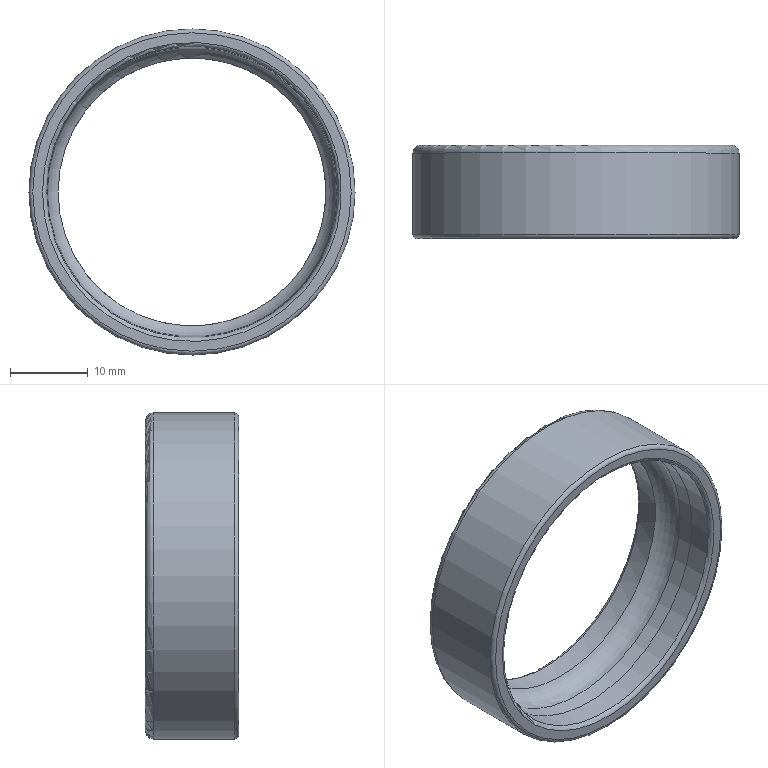Part | STEP file | BK-20_id1310_x_t | 1 solid | 11 faces | box 42 x 12 x 42 mm | volume 4062 mm3 | torus 5 | cylinder 3 | plane 2 | cone 1 | commonest cylinder face diameters 34.5 x1 37.5 x1 42 x1
STEP:
#1=CARTESIAN_POINT('',(0.,0.,0.));
#2=DIRECTION('',(0.,0.,1.));
#3=DIRECTION('',(1.,0.,0.));
#4=AXIS2_PLACEMENT_3D('',#1,#2,#3);
#5=CARTESIAN_POINT('',(-249.75,533.436,-165.5));
#6=VERTEX_POINT('',#5);
#7=CARTESIAN_POINT('',(-287.25,533.436,-165.5));
#8=VERTEX_POINT('',#7);
#9=CARTESIAN_POINT('',(-268.5,533.436,-165.5));
#10=DIRECTION('',(0.,-1.,0.));
#11=DIRECTION('',(-1.,0.,0.));
#12=AXIS2_PLACEMENT_3D('',#9,#10,#11);
#13=CIRCLE('',#12,18.75);
#14=CARTESIAN_POINT('',(-268.5,533.436,-165.5));
#15=DIRECTION('',(0.,-1.,0.));
#16=DIRECTION('',(1.,0.,0.));
#17=AXIS2_PLACEMENT_3D('',#14,#15,#16);
#18=CONICAL_SURFACE('',#17,18.75,0.05236);
#19=CARTESIAN_POINT('',(-3.142,0.));
#20=DIRECTION('',(1.,0.));
#21=VECTOR('',#20,1.);
#22=LINE('',#19,#21);
#23=(GEOMETRIC_REPRESENTATION_CONTEXT(2)PARAMETRIC_REPRESENTATION_CONTEXT()REPRESENTATION_CONTEXT('',''));
#24=DEFINITIONAL_REPRESENTATION('',(#22),#23);
#25=PCURVE('',#18,#24);
#26=CARTESIAN_POINT('',(-268.5,604.298,-165.5));
#27=DIRECTION('',(0.,1.,0.));
#28=DIRECTION('',(-1.,0.,0.));
#29=AXIS2_PLACEMENT_3D('',#26,#27,#28);
#30=CYLINDRICAL_SURFACE('',#29,18.75);
#31=CARTESIAN_POINT('',(12.566,-70.863));
#32=DIRECTION('',(-1.,0.));
#33=VECTOR('',#32,1.);
#34=LINE('',#31,#33);
#35=(GEOMETRIC_REPRESENTATION_CONTEXT(2)PARAMETRIC_REPRESENTATION_CONTEXT()REPRESENTATION_CONTEXT('',''));
#36=DEFINITIONAL_REPRESENTATION('',(#34),#35);
#37=PCURVE('',#30,#36);
#38=SURFACE_CURVE('',#13,(#25,#37),.PCURVE_S1.);
#39=EDGE_CURVE('',#6,#8,#38,.T.);
#40=ORIENTED_EDGE('',*,*,#39,.F.);
#41=CARTESIAN_POINT('',(-249.857,535.484,-165.5));
#42=VERTEX_POINT('',#41);
#43=CARTESIAN_POINT('',(-249.857,535.484,-165.5));
#44=CARTESIAN_POINT('',(-249.75,533.436,-165.5));
#45=B_SPLINE_CURVE_WITH_KNOTS('',1,(#43,#44),.UNSPECIFIED.,.F.,.F.,(2,2),(-2.051,0.),.PIECEWISE_BEZIER_KNOTS.);
#46=CARTESIAN_POINT('',(0.,0.));
#47=DIRECTION('',(0.,1.));
#48=VECTOR('',#47,1.);
#49=LINE('',#46,#48);
#50=(GEOMETRIC_REPRESENTATION_CONTEXT(2)PARAMETRIC_REPRESENTATION_CONTEXT()REPRESENTATION_CONTEXT('',''));
#51=DEFINITIONAL_REPRESENTATION('',(#49),#50);
#52=PCURVE('',#18,#51);
#53=CARTESIAN_POINT('',(6.283,0.));
#54=DIRECTION('',(0.,1.));
#55=VECTOR('',#54,1.);
#56=LINE('',#53,#55);
#57=(GEOMETRIC_REPRESENTATION_CONTEXT(2)PARAMETRIC_REPRESENTATION_CONTEXT()REPRESENTATION_CONTEXT('',''));
#58=DEFINITIONAL_REPRESENTATION('',(#56),#57);
#59=PCURVE('',#18,#58);
#60=SEAM_CURVE('',#45,(#52,#59),.PCURVE_S1.);
#61=EDGE_CURVE('',#42,#6,#60,.T.);
#62=ORIENTED_EDGE('',*,*,#61,.F.);
#63=CARTESIAN_POINT('',(-287.143,535.484,-165.5));
#64=VERTEX_POINT('',#63);
#65=CARTESIAN_POINT('',(-268.5,535.484,-165.5));
#66=DIRECTION('',(0.,-1.,0.));
#67=DIRECTION('',(1.,0.,0.));
#68=AXIS2_PLACEMENT_3D('',#65,#66,#67);
#69=CIRCLE('',#68,18.643);
#70=CARTESIAN_POINT('',(0.,-2.048));
#71=DIRECTION('',(1.,0.));
#72=VECTOR('',#71,1.);
#73=LINE('',#70,#72);
#74=(GEOMETRIC_REPRESENTATION_CONTEXT(2)PARAMETRIC_REPRESENTATION_CONTEXT()REPRESENTATION_CONTEXT('',''));
#75=DEFINITIONAL_REPRESENTATION('',(#73),#74);
#76=PCURVE('',#18,#75);
#77=CARTESIAN_POINT('',(-268.5,535.936,-165.5));
#78=DIRECTION('',(0.,1.,0.));
#79=DIRECTION('',(-1.,0.,0.));
#80=AXIS2_PLACEMENT_3D('',#77,#78,#79);
#81=TOROIDAL_SURFACE('',#80,15.5,3.175);
#82=CARTESIAN_POINT('',(3.142,6.14));
#83=DIRECTION('',(-1.,0.));
#84=VECTOR('',#83,1.);
#85=LINE('',#82,#84);
#86=(GEOMETRIC_REPRESENTATION_CONTEXT(2)PARAMETRIC_REPRESENTATION_CONTEXT()REPRESENTATION_CONTEXT('',''));
#87=DEFINITIONAL_REPRESENTATION('',(#85),#86);
#88=PCURVE('',#81,#87);
#89=SURFACE_CURVE('',#69,(#76,#88),.PCURVE_S1.);
#90=EDGE_CURVE('',#42,#64,#89,.T.);
#91=ORIENTED_EDGE('',*,*,#90,.T.);
#92=CARTESIAN_POINT('',(-268.5,535.484,-165.5));
#93=DIRECTION('',(0.,-1.,0.));
#94=DIRECTION('',(1.,0.,0.));
#95=AXIS2_PLACEMENT_3D('',#92,#93,#94);
#96=CIRCLE('',#95,18.643);
#97=CARTESIAN_POINT('',(0.,-2.048));
#98=DIRECTION('',(1.,0.));
#99=VECTOR('',#98,1.);
#100=LINE('',#97,#99);
#101=(GEOMETRIC_REPRESENTATION_CONTEXT(2)PARAMETRIC_REPRESENTATION_CONTEXT()REPRESENTATION_CONTEXT('',''));
#102=DEFINITIONAL_REPRESENTATION('',(#100),#101);
#103=PCURVE('',#18,#102);
#104=CARTESIAN_POINT('',(9.425,6.14));
#105=DIRECTION('',(-1.,0.));
#106=VECTOR('',#105,1.);
#107=LINE('',#104,#106);
#108=(GEOMETRIC_REPRESENTATION_CONTEXT(2)PARAMETRIC_REPRESENTATION_CONTEXT()REPRESENTATION_CONTEXT('',''));
#109=DEFINITIONAL_REPRESENTATION('',(#107),#108);
#110=PCURVE('',#81,#109);
#111=SURFACE_CURVE('',#96,(#103,#110),.PCURVE_S1.);
#112=EDGE_CURVE('',#64,#42,#111,.T.);
#113=ORIENTED_EDGE('',*,*,#112,.T.);
#114=ORIENTED_EDGE('',*,*,#61,.T.);
#115=CARTESIAN_POINT('',(-268.5,533.436,-165.5));
#116=DIRECTION('',(0.,-1.,0.));
#117=DIRECTION('',(-1.,0.,0.));
#118=AXIS2_PLACEMENT_3D('',#115,#116,#117);
#119=CIRCLE('',#118,18.75);
#120=CARTESIAN_POINT('',(3.142,0.));
#121=DIRECTION('',(1.,0.));
#122=VECTOR('',#121,1.);
#123=LINE('',#120,#122);
#124=(GEOMETRIC_REPRESENTATION_CONTEXT(2)PARAMETRIC_REPRESENTATION_CONTEXT()REPRESENTATION_CONTEXT('',''));
#125=DEFINITIONAL_REPRESENTATION('',(#123),#124);
#126=PCURVE('',#18,#125);
#127=CARTESIAN_POINT('',(6.283,-70.863));
#128=DIRECTION('',(-1.,0.));
#129=VECTOR('',#128,1.);
#130=LINE('',#127,#129);
#131=(GEOMETRIC_REPRESENTATION_CONTEXT(2)PARAMETRIC_REPRESENTATION_CONTEXT()REPRESENTATION_CONTEXT('',''));
#132=DEFINITIONAL_REPRESENTATION('',(#130),#131);
#133=PCURVE('',#30,#132);
#134=SURFACE_CURVE('',#119,(#126,#133),.PCURVE_S1.);
#135=EDGE_CURVE('',#8,#6,#134,.T.);
#136=ORIENTED_EDGE('',*,*,#135,.F.);
#137=EDGE_LOOP('',(#40,#62,#91,#113,#114,#136));
#138=FACE_BOUND('',#137,.F.);
#139=ADVANCED_FACE('',(#138),#18,.F.);
#140=ORIENTED_EDGE('',*,*,#112,.F.);
#141=CARTESIAN_POINT('',(-285.75,538.585,-165.5));
#142=VERTEX_POINT('',#141);
#143=CARTESIAN_POINT('',(-287.143,535.484,-165.5));
#144=CARTESIAN_POINT('',(-287.228,536.075,-165.5));
#145=CARTESIAN_POINT('',(-287.179,536.686,-165.5));
#146=CARTESIAN_POINT('',(-286.991,537.279,-165.5));
#147=CARTESIAN_POINT('',(-286.673,537.813,-165.5));
#148=CARTESIAN_POINT('',(-286.249,538.255,-165.5));
#149=CARTESIAN_POINT('',(-285.75,538.585,-165.5));
#150=B_SPLINE_CURVE_WITH_KNOTS('',6,(#143,#144,#145,#146,#147,#148,#149),.UNSPECIFIED.,.F.,.F.,(7,7),(6.14,7.27),.PIECEWISE_BEZIER_KNOTS.);
#151=CARTESIAN_POINT('',(6.283,0.));
#152=DIRECTION('',(0.,1.));
#153=VECTOR('',#152,1.);
#154=LINE('',#151,#153);
#155=(GEOMETRIC_REPRESENTATION_CONTEXT(2)PARAMETRIC_REPRESENTATION_CONTEXT()REPRESENTATION_CONTEXT('',''));
#156=DEFINITIONAL_REPRESENTATION('',(#154),#155);
#157=PCURVE('',#81,#156);
#158=CARTESIAN_POINT('',(0.,0.));
#159=DIRECTION('',(0.,1.));
#160=VECTOR('',#159,1.);
#161=LINE('',#158,#160);
#162=(GEOMETRIC_REPRESENTATION_CONTEXT(2)PARAMETRIC_REPRESENTATION_CONTEXT()REPRESENTATION_CONTEXT('',''));
#163=DEFINITIONAL_REPRESENTATION('',(#161),#162);
#164=PCURVE('',#81,#163);
#165=SEAM_CURVE('',#150,(#157,#164),.PCURVE_S1.);
#166=EDGE_CURVE('',#64,#142,#165,.T.);
#167=ORIENTED_EDGE('',*,*,#166,.T.);
#168=CARTESIAN_POINT('',(-268.5,538.585,-165.5));
#169=DIRECTION('',(0.,1.,0.));
#170=DIRECTION('',(-1.,0.,0.));
#171=AXIS2_PLACEMENT_3D('',#168,#169,#170);
#172=CIRCLE('',#171,17.25);
#173=CARTESIAN_POINT('',(0.,7.27));
#174=DIRECTION('',(1.,0.));
#175=VECTOR('',#174,1.);
#176=LINE('',#173,#175);
#177=(GEOMETRIC_REPRESENTATION_CONTEXT(2)PARAMETRIC_REPRESENTATION_CONTEXT()REPRESENTATION_CONTEXT('',''));
#178=DEFINITIONAL_REPRESENTATION('',(#176),#177);
#179=PCURVE('',#81,#178);
#180=CARTESIAN_POINT('',(-268.5,604.298,-165.5));
#181=DIRECTION('',(0.,1.,0.));
#182=DIRECTION('',(-1.,0.,0.));
#183=AXIS2_PLACEMENT_3D('',#180,#181,#182);
#184=CYLINDRICAL_SURFACE('',#183,17.25);
#185=CARTESIAN_POINT('',(0.,-65.713));
#186=DIRECTION('',(1.,0.));
#187=VECTOR('',#186,1.);
#188=LINE('',#185,#187);
#189=(GEOMETRIC_REPRESENTATION_CONTEXT(2)PARAMETRIC_REPRESENTATION_CONTEXT()REPRESENTATION_CONTEXT('',''));
#190=DEFINITIONAL_REPRESENTATION('',(#188),#189);
#191=PCURVE('',#184,#190);
#192=SURFACE_CURVE('',#172,(#179,#191),.PCURVE_S1.);
#193=EDGE_CURVE('',#142,#142,#192,.T.);
#194=ORIENTED_EDGE('',*,*,#193,.F.);
#195=ORIENTED_EDGE('',*,*,#166,.F.);
#196=ORIENTED_EDGE('',*,*,#90,.F.);
#197=EDGE_LOOP('',(#140,#167,#194,#195,#196));
#198=FACE_BOUND('',#197,.F.);
#199=ADVANCED_FACE('',(#198),#81,.F.);
#200=ORIENTED_EDGE('',*,*,#39,.T.);
#201=ORIENTED_EDGE('',*,*,#135,.T.);
#202=CARTESIAN_POINT('',(-249.75,530.436,-165.5));
#203=VERTEX_POINT('',#202);
#204=CARTESIAN_POINT('',(-249.75,530.436,-165.5));
#205=CARTESIAN_POINT('',(-249.75,533.436,-165.5));
#206=B_SPLINE_CURVE_WITH_KNOTS('',1,(#204,#205),.UNSPECIFIED.,.F.,.F.,(2,2),(-73.863,-70.863),.PIECEWISE_BEZIER_KNOTS.);
#207=CARTESIAN_POINT('',(3.142,0.));
#208=DIRECTION('',(0.,1.));
#209=VECTOR('',#208,1.);
#210=LINE('',#207,#209);
#211=(GEOMETRIC_REPRESENTATION_CONTEXT(2)PARAMETRIC_REPRESENTATION_CONTEXT()REPRESENTATION_CONTEXT('',''));
#212=DEFINITIONAL_REPRESENTATION('',(#210),#211);
#213=PCURVE('',#30,#212);
#214=CARTESIAN_POINT('',(9.425,0.));
#215=DIRECTION('',(0.,1.));
#216=VECTOR('',#215,1.);
#217=LINE('',#214,#216);
#218=(GEOMETRIC_REPRESENTATION_CONTEXT(2)PARAMETRIC_REPRESENTATION_CONTEXT()REPRESENTATION_CONTEXT('',''));
#219=DEFINITIONAL_REPRESENTATION('',(#217),#218);
#220=PCURVE('',#30,#219);
#221=SEAM_CURVE('',#206,(#213,#220),.PCURVE_S1.);
#222=EDGE_CURVE('',#203,#6,#221,.T.);
#223=ORIENTED_EDGE('',*,*,#222,.F.);
#224=CARTESIAN_POINT('',(-287.25,530.436,-165.5));
#225=VERTEX_POINT('',#224);
#226=CARTESIAN_POINT('',(-268.5,530.436,-165.5));
#227=DIRECTION('',(0.,1.,0.));
#228=DIRECTION('',(1.,0.,0.));
#229=AXIS2_PLACEMENT_3D('',#226,#227,#228);
#230=CIRCLE('',#229,18.75);
#231=CARTESIAN_POINT('',(3.142,-73.863));
#232=DIRECTION('',(1.,0.));
#233=VECTOR('',#232,1.);
#234=LINE('',#231,#233);
#235=(GEOMETRIC_REPRESENTATION_CONTEXT(2)PARAMETRIC_REPRESENTATION_CONTEXT()REPRESENTATION_CONTEXT('',''));
#236=DEFINITIONAL_REPRESENTATION('',(#234),#235);
#237=PCURVE('',#30,#236);
#238=CARTESIAN_POINT('',(-268.5,530.436,-165.5));
#239=DIRECTION('',(0.,1.,0.));
#240=DIRECTION('',(-1.,0.,0.));
#241=AXIS2_PLACEMENT_3D('',#238,#239,#240);
#242=TOROIDAL_SURFACE('',#241,19.25,0.5);
#243=CARTESIAN_POINT('',(3.142,3.142));
#244=DIRECTION('',(1.,0.));
#245=VECTOR('',#244,1.);
#246=LINE('',#243,#245);
#247=(GEOMETRIC_REPRESENTATION_CONTEXT(2)PARAMETRIC_REPRESENTATION_CONTEXT()REPRESENTATION_CONTEXT('',''));
#248=DEFINITIONAL_REPRESENTATION('',(#246),#247);
#249=PCURVE('',#242,#248);
#250=SURFACE_CURVE('',#230,(#237,#249),.PCURVE_S1.);
#251=EDGE_CURVE('',#203,#225,#250,.T.);
#252=ORIENTED_EDGE('',*,*,#251,.T.);
#253=CARTESIAN_POINT('',(-268.5,530.436,-165.5));
#254=DIRECTION('',(0.,1.,0.));
#255=DIRECTION('',(1.,0.,0.));
#256=AXIS2_PLACEMENT_3D('',#253,#254,#255);
#257=CIRCLE('',#256,18.75);
#258=CARTESIAN_POINT('',(3.142,-73.863));
#259=DIRECTION('',(1.,0.));
#260=VECTOR('',#259,1.);
#261=LINE('',#258,#260);
#262=(GEOMETRIC_REPRESENTATION_CONTEXT(2)PARAMETRIC_REPRESENTATION_CONTEXT()REPRESENTATION_CONTEXT('',''));
#263=DEFINITIONAL_REPRESENTATION('',(#261),#262);
#264=PCURVE('',#30,#263);
#265=CARTESIAN_POINT('',(-3.142,3.142));
#266=DIRECTION('',(1.,0.));
#267=VECTOR('',#266,1.);
#268=LINE('',#265,#267);
#269=(GEOMETRIC_REPRESENTATION_CONTEXT(2)PARAMETRIC_REPRESENTATION_CONTEXT()REPRESENTATION_CONTEXT('',''));
#270=DEFINITIONAL_REPRESENTATION('',(#268),#269);
#271=PCURVE('',#242,#270);
#272=SURFACE_CURVE('',#257,(#264,#271),.PCURVE_S1.);
#273=EDGE_CURVE('',#225,#203,#272,.T.);
#274=ORIENTED_EDGE('',*,*,#273,.T.);
#275=ORIENTED_EDGE('',*,*,#222,.T.);
#276=EDGE_LOOP('',(#200,#201,#223,#252,#274,#275));
#277=FACE_BOUND('',#276,.F.);
#278=ADVANCED_FACE('',(#277),#30,.F.);
#279=CARTESIAN_POINT('',(-251.25,541.436,-165.5));
#280=VERTEX_POINT('',#279);
#281=CARTESIAN_POINT('',(-285.75,541.436,-165.5));
#282=VERTEX_POINT('',#281);
#283=CARTESIAN_POINT('',(-268.5,541.436,-165.5));
#284=DIRECTION('',(0.,-1.,0.));
#285=DIRECTION('',(1.,0.,0.));
#286=AXIS2_PLACEMENT_3D('',#283,#284,#285);
#287=CIRCLE('',#286,17.25);
#288=CARTESIAN_POINT('',(3.142,-62.863));
#289=DIRECTION('',(-1.,0.));
#290=VECTOR('',#289,1.);
#291=LINE('',#288,#290);
#292=(GEOMETRIC_REPRESENTATION_CONTEXT(2)PARAMETRIC_REPRESENTATION_CONTEXT()REPRESENTATION_CONTEXT('',''));
#293=DEFINITIONAL_REPRESENTATION('',(#291),#292);
#294=PCURVE('',#184,#293);
#295=CARTESIAN_POINT('',(-268.5,541.436,-165.5));
#296=DIRECTION('',(0.,1.,0.));
#297=DIRECTION('',(-1.,0.,0.));
#298=AXIS2_PLACEMENT_3D('',#295,#296,#297);
#299=TOROIDAL_SURFACE('',#298,17.75,0.5);
#300=CARTESIAN_POINT('',(3.142,9.425));
#301=DIRECTION('',(-1.,0.));
#302=VECTOR('',#301,1.);
#303=LINE('',#300,#302);
#304=(GEOMETRIC_REPRESENTATION_CONTEXT(2)PARAMETRIC_REPRESENTATION_CONTEXT()REPRESENTATION_CONTEXT('',''));
#305=DEFINITIONAL_REPRESENTATION('',(#303),#304);
#306=PCURVE('',#299,#305);
#307=SURFACE_CURVE('',#287,(#294,#306),.PCURVE_S1.);
#308=EDGE_CURVE('',#280,#282,#307,.T.);
#309=ORIENTED_EDGE('',*,*,#308,.T.);
#310=CARTESIAN_POINT('',(-285.75,538.585,-165.5));
#311=CARTESIAN_POINT('',(-285.75,541.436,-165.5));
#312=B_SPLINE_CURVE_WITH_KNOTS('',1,(#310,#311),.UNSPECIFIED.,.F.,.F.,(2,2),(-65.713,-62.863),.PIECEWISE_BEZIER_KNOTS.);
#313=CARTESIAN_POINT('',(0.,0.));
#314=DIRECTION('',(0.,1.));
#315=VECTOR('',#314,1.);
#316=LINE('',#313,#315);
#317=(GEOMETRIC_REPRESENTATION_CONTEXT(2)PARAMETRIC_REPRESENTATION_CONTEXT()REPRESENTATION_CONTEXT('',''));
#318=DEFINITIONAL_REPRESENTATION('',(#316),#317);
#319=PCURVE('',#184,#318);
#320=CARTESIAN_POINT('',(6.283,0.));
#321=DIRECTION('',(0.,1.));
#322=VECTOR('',#321,1.);
#323=LINE('',#320,#322);
#324=(GEOMETRIC_REPRESENTATION_CONTEXT(2)PARAMETRIC_REPRESENTATION_CONTEXT()REPRESENTATION_CONTEXT('',''));
#325=DEFINITIONAL_REPRESENTATION('',(#323),#324);
#326=PCURVE('',#184,#325);
#327=SEAM_CURVE('',#312,(#319,#326),.PCURVE_S1.);
#328=EDGE_CURVE('',#142,#282,#327,.T.);
#329=ORIENTED_EDGE('',*,*,#328,.F.);
#330=ORIENTED_EDGE('',*,*,#193,.T.);
#331=ORIENTED_EDGE('',*,*,#328,.T.);
#332=CARTESIAN_POINT('',(-268.5,541.436,-165.5));
#333=DIRECTION('',(0.,-1.,0.));
#334=DIRECTION('',(1.,0.,0.));
#335=AXIS2_PLACEMENT_3D('',#332,#333,#334);
#336=CIRCLE('',#335,17.25);
#337=CARTESIAN_POINT('',(9.425,-62.863));
#338=DIRECTION('',(-1.,0.));
#339=VECTOR('',#338,1.);
#340=LINE('',#337,#339);
#341=(GEOMETRIC_REPRESENTATION_CONTEXT(2)PARAMETRIC_REPRESENTATION_CONTEXT()REPRESENTATION_CONTEXT('',''));
#342=DEFINITIONAL_REPRESENTATION('',(#340),#341);
#343=PCURVE('',#184,#342);
#344=CARTESIAN_POINT('',(9.425,9.425));
#345=DIRECTION('',(-1.,0.));
#346=VECTOR('',#345,1.);
#347=LINE('',#344,#346);
#348=(GEOMETRIC_REPRESENTATION_CONTEXT(2)PARAMETRIC_REPRESENTATION_CONTEXT()REPRESENTATION_CONTEXT('',''));
#349=DEFINITIONAL_REPRESENTATION('',(#347),#348);
#350=PCURVE('',#299,#349);
#351=SURFACE_CURVE('',#336,(#343,#350),.PCURVE_S1.);
#352=EDGE_CURVE('',#282,#280,#351,.T.);
#353=ORIENTED_EDGE('',*,*,#352,.T.);
#354=EDGE_LOOP('',(#309,#329,#330,#331,#353));
#355=FACE_BOUND('',#354,.F.);
#356=ADVANCED_FACE('',(#355),#184,.F.);
#357=ORIENTED_EDGE('',*,*,#251,.T.);
#358=CARTESIAN_POINT('',(-287.75,529.936,-165.5));
#359=VERTEX_POINT('',#358);
#360=CARTESIAN_POINT('',(-287.25,530.436,-165.5));
#361=CARTESIAN_POINT('',(-287.25,530.302,-165.5));
#362=CARTESIAN_POINT('',(-287.293,530.172,-165.5));
#363=CARTESIAN_POINT('',(-287.374,530.06,-165.5));
#364=CARTESIAN_POINT('',(-287.486,529.978,-165.5));
#365=CARTESIAN_POINT('',(-287.616,529.936,-165.5));
#366=CARTESIAN_POINT('',(-287.75,529.936,-165.5));
#367=(BOUNDED_CURVE()B_SPLINE_CURVE(6,(#360,#361,#362,#363,#364,#365,#366),.UNSPECIFIED.,.F.,.F.)B_SPLINE_CURVE_WITH_KNOTS((7,7),(3.142,4.712),.PIECEWISE_BEZIER_KNOTS.)CURVE()GEOMETRIC_REPRESENTATION_ITEM()RATIONAL_B_SPLINE_CURVE((1.031,1.01,0.9979,0.994,0.9979,1.01,1.031))REPRESENTATION_ITEM(''));
#368=CARTESIAN_POINT('',(6.283,0.));
#369=DIRECTION('',(0.,1.));
#370=VECTOR('',#369,1.);
#371=LINE('',#368,#370);
#372=(GEOMETRIC_REPRESENTATION_CONTEXT(2)PARAMETRIC_REPRESENTATION_CONTEXT()REPRESENTATION_CONTEXT('',''));
#373=DEFINITIONAL_REPRESENTATION('',(#371),#372);
#374=PCURVE('',#242,#373);
#375=CARTESIAN_POINT('',(0.,0.));
#376=DIRECTION('',(0.,1.));
#377=VECTOR('',#376,1.);
#378=LINE('',#375,#377);
#379=(GEOMETRIC_REPRESENTATION_CONTEXT(2)PARAMETRIC_REPRESENTATION_CONTEXT()REPRESENTATION_CONTEXT('',''));
#380=DEFINITIONAL_REPRESENTATION('',(#378),#379);
#381=PCURVE('',#242,#380);
#382=SEAM_CURVE('',#367,(#374,#381),.PCURVE_S1.);
#383=EDGE_CURVE('',#225,#359,#382,.T.);
#384=ORIENTED_EDGE('',*,*,#383,.T.);
#385=CARTESIAN_POINT('',(-268.5,529.936,-165.5));
#386=DIRECTION('',(0.,-1.,0.));
#387=DIRECTION('',(-1.,0.,0.));
#388=AXIS2_PLACEMENT_3D('',#385,#386,#387);
#389=CIRCLE('',#388,19.25);
#390=CARTESIAN_POINT('',(6.283,4.712));
#391=DIRECTION('',(-1.,0.));
#392=VECTOR('',#391,1.);
#393=LINE('',#390,#392);
#394=(GEOMETRIC_REPRESENTATION_CONTEXT(2)PARAMETRIC_REPRESENTATION_CONTEXT()REPRESENTATION_CONTEXT('',''));
#395=DEFINITIONAL_REPRESENTATION('',(#393),#394);
#396=PCURVE('',#242,#395);
#397=CARTESIAN_POINT('',(-268.5,529.936,-146.25));
#398=DIRECTION('',(0.,1.,0.));
#399=DIRECTION('',(-1.,0.,0.));
#400=AXIS2_PLACEMENT_3D('',#397,#398,#399);
#401=PLANE('',#400);
#402=CARTESIAN_POINT('',(19.25,-19.25));
#403=CARTESIAN_POINT('',(19.25,-52.592));
#404=CARTESIAN_POINT('',(-9.625,-35.921));
#405=CARTESIAN_POINT('',(-38.5,-19.25));
#406=CARTESIAN_POINT('',(-9.625,-2.579));
#407=CARTESIAN_POINT('',(19.25,14.092));
#408=CARTESIAN_POINT('',(19.25,-19.25));
#409=(BOUNDED_CURVE()B_SPLINE_CURVE(2,(#402,#403,#404,#405,#406,#407,#408),.UNSPECIFIED.,.T.,.F.)B_SPLINE_CURVE_WITH_KNOTS((1,2,2,2,2,1),(-2.094,0.,2.094,4.189,6.283,8.378),.UNSPECIFIED.)CURVE()GEOMETRIC_REPRESENTATION_ITEM()RATIONAL_B_SPLINE_CURVE((1.,0.5,1.,0.5,1.,0.5,1.))REPRESENTATION_ITEM(''));
#410=(GEOMETRIC_REPRESENTATION_CONTEXT(2)PARAMETRIC_REPRESENTATION_CONTEXT()REPRESENTATION_CONTEXT('',''));
#411=DEFINITIONAL_REPRESENTATION('',(#409),#410);
#412=PCURVE('',#401,#411);
#413=SURFACE_CURVE('',#389,(#396,#412),.PCURVE_S1.);
#414=EDGE_CURVE('',#359,#359,#413,.T.);
#415=ORIENTED_EDGE('',*,*,#414,.T.);
#416=ORIENTED_EDGE('',*,*,#383,.F.);
#417=ORIENTED_EDGE('',*,*,#273,.T.);
#418=EDGE_LOOP('',(#357,#384,#415,#416,#417));
#419=FACE_BOUND('',#418,.T.);
#420=ADVANCED_FACE('',(#419),#242,.T.);
#421=CARTESIAN_POINT('',(-286.25,541.936,-165.5));
#422=VERTEX_POINT('',#421);
#423=CARTESIAN_POINT('',(-268.5,541.936,-165.5));
#424=DIRECTION('',(0.,1.,0.));
#425=DIRECTION('',(-1.,0.,0.));
#426=AXIS2_PLACEMENT_3D('',#423,#424,#425);
#427=CIRCLE('',#426,17.75);
#428=CARTESIAN_POINT('',(0.,7.854));
#429=DIRECTION('',(1.,0.));
#430=VECTOR('',#429,1.);
#431=LINE('',#428,#430);
#432=(GEOMETRIC_REPRESENTATION_CONTEXT(2)PARAMETRIC_REPRESENTATION_CONTEXT()REPRESENTATION_CONTEXT('',''));
#433=DEFINITIONAL_REPRESENTATION('',(#431),#432);
#434=PCURVE('',#299,#433);
#435=CARTESIAN_POINT('',(-268.5,541.936,-145.5));
#436=DIRECTION('',(0.,-1.,0.));
#437=DIRECTION('',(1.,0.,0.));
#438=AXIS2_PLACEMENT_3D('',#435,#436,#437);
#439=PLANE('',#438);
#440=CARTESIAN_POINT('',(-17.75,-20.));
#441=CARTESIAN_POINT('',(-17.75,10.744));
#442=CARTESIAN_POINT('',(8.875,-4.628));
#443=CARTESIAN_POINT('',(35.5,-20.));
#444=CARTESIAN_POINT('',(8.875,-35.372));
#445=CARTESIAN_POINT('',(-17.75,-50.744));
#446=CARTESIAN_POINT('',(-17.75,-20.));
#447=(BOUNDED_CURVE()B_SPLINE_CURVE(2,(#440,#441,#442,#443,#444,#445,#446),.UNSPECIFIED.,.T.,.F.)B_SPLINE_CURVE_WITH_KNOTS((1,2,2,2,2,1),(-2.094,0.,2.094,4.189,6.283,8.378),.UNSPECIFIED.)CURVE()GEOMETRIC_REPRESENTATION_ITEM()RATIONAL_B_SPLINE_CURVE((1.,0.5,1.,0.5,1.,0.5,1.))REPRESENTATION_ITEM(''));
#448=(GEOMETRIC_REPRESENTATION_CONTEXT(2)PARAMETRIC_REPRESENTATION_CONTEXT()REPRESENTATION_CONTEXT('',''));
#449=DEFINITIONAL_REPRESENTATION('',(#447),#448);
#450=PCURVE('',#439,#449);
#451=SURFACE_CURVE('',#427,(#434,#450),.PCURVE_S1.);
#452=EDGE_CURVE('',#422,#422,#451,.T.);
#453=ORIENTED_EDGE('',*,*,#452,.T.);
#454=CARTESIAN_POINT('',(-286.25,541.936,-165.5));
#455=CARTESIAN_POINT('',(-286.116,541.936,-165.5));
#456=CARTESIAN_POINT('',(-285.986,541.893,-165.5));
#457=CARTESIAN_POINT('',(-285.874,541.812,-165.5));
#458=CARTESIAN_POINT('',(-285.793,541.699,-165.5));
#459=CARTESIAN_POINT('',(-285.75,541.569,-165.5));
#460=CARTESIAN_POINT('',(-285.75,541.436,-165.5));
#461=(BOUNDED_CURVE()B_SPLINE_CURVE(6,(#454,#455,#456,#457,#458,#459,#460),.UNSPECIFIED.,.F.,.F.)B_SPLINE_CURVE_WITH_KNOTS((7,7),(1.571,3.142),.PIECEWISE_BEZIER_KNOTS.)CURVE()GEOMETRIC_REPRESENTATION_ITEM()RATIONAL_B_SPLINE_CURVE((1.031,1.01,0.9979,0.994,0.9979,1.01,1.031))REPRESENTATION_ITEM(''));
#462=CARTESIAN_POINT('',(6.283,6.283));
#463=DIRECTION('',(0.,1.));
#464=VECTOR('',#463,1.);
#465=LINE('',#462,#464);
#466=(GEOMETRIC_REPRESENTATION_CONTEXT(2)PARAMETRIC_REPRESENTATION_CONTEXT()REPRESENTATION_CONTEXT('',''));
#467=DEFINITIONAL_REPRESENTATION('',(#465),#466);
#468=PCURVE('',#299,#467);
#469=CARTESIAN_POINT('',(0.,6.283));
#470=DIRECTION('',(0.,1.));
#471=VECTOR('',#470,1.);
#472=LINE('',#469,#471);
#473=(GEOMETRIC_REPRESENTATION_CONTEXT(2)PARAMETRIC_REPRESENTATION_CONTEXT()REPRESENTATION_CONTEXT('',''));
#474=DEFINITIONAL_REPRESENTATION('',(#472),#473);
#475=PCURVE('',#299,#474);
#476=SEAM_CURVE('',#461,(#468,#475),.PCURVE_S1.);
#477=EDGE_CURVE('',#422,#282,#476,.T.);
#478=ORIENTED_EDGE('',*,*,#477,.T.);
#479=ORIENTED_EDGE('',*,*,#352,.T.);
#480=ORIENTED_EDGE('',*,*,#308,.T.);
#481=ORIENTED_EDGE('',*,*,#477,.F.);
#482=EDGE_LOOP('',(#453,#478,#479,#480,#481));
#483=FACE_BOUND('',#482,.T.);
#484=ADVANCED_FACE('',(#483),#299,.T.);
#485=CARTESIAN_POINT('',(-289.,529.936,-165.5));
#486=VERTEX_POINT('',#485);
#487=CARTESIAN_POINT('',(-268.5,529.936,-165.5));
#488=DIRECTION('',(0.,1.,0.));
#489=DIRECTION('',(-1.,0.,0.));
#490=AXIS2_PLACEMENT_3D('',#487,#488,#489);
#491=CIRCLE('',#490,20.5);
#492=CARTESIAN_POINT('',(0.,-19.25));
#493=DIRECTION('',(1.,0.));
#494=AXIS2_PLACEMENT_2D('',#492,#493);
#495=CIRCLE('',#494,20.5);
#496=(GEOMETRIC_REPRESENTATION_CONTEXT(2)PARAMETRIC_REPRESENTATION_CONTEXT()REPRESENTATION_CONTEXT('',''));
#497=DEFINITIONAL_REPRESENTATION('',(#495),#496);
#498=PCURVE('',#401,#497);
#499=CARTESIAN_POINT('',(-268.5,530.436,-165.5));
#500=DIRECTION('',(0.,1.,0.));
#501=DIRECTION('',(-1.,0.,0.));
#502=AXIS2_PLACEMENT_3D('',#499,#500,#501);
#503=TOROIDAL_SURFACE('',#502,20.5,0.5);
#504=CARTESIAN_POINT('',(0.,4.712));
#505=DIRECTION('',(1.,0.));
#506=VECTOR('',#505,1.);
#507=LINE('',#504,#506);
#508=(GEOMETRIC_REPRESENTATION_CONTEXT(2)PARAMETRIC_REPRESENTATION_CONTEXT()REPRESENTATION_CONTEXT('',''));
#509=DEFINITIONAL_REPRESENTATION('',(#507),#508);
#510=PCURVE('',#503,#509);
#511=SURFACE_CURVE('',#491,(#498,#510),.PCURVE_S1.);
#512=EDGE_CURVE('',#486,#486,#511,.T.);
#513=ORIENTED_EDGE('',*,*,#512,.F.);
#514=EDGE_LOOP('',(#513));
#515=FACE_BOUND('',#514,.T.);
#516=ORIENTED_EDGE('',*,*,#414,.F.);
#517=EDGE_LOOP('',(#516));
#518=FACE_BOUND('',#517,.T.);
#519=ADVANCED_FACE('',(#515,#518),#401,.F.);
#520=ORIENTED_EDGE('',*,*,#452,.F.);
#521=EDGE_LOOP('',(#520));
#522=FACE_BOUND('',#521,.T.);
#523=CARTESIAN_POINT('',(-288.5,541.936,-165.5));
#524=VERTEX_POINT('',#523);
#525=CARTESIAN_POINT('',(-268.5,541.936,-165.5));
#526=DIRECTION('',(0.,-1.,0.));
#527=DIRECTION('',(-1.,0.,0.));
#528=AXIS2_PLACEMENT_3D('',#525,#526,#527);
#529=CIRCLE('',#528,20.);
#530=CARTESIAN_POINT('',(0.,-20.));
#531=DIRECTION('',(-1.,0.));
#532=AXIS2_PLACEMENT_2D('',#530,#531);
#533=CIRCLE('',#532,20.);
#534=(GEOMETRIC_REPRESENTATION_CONTEXT(2)PARAMETRIC_REPRESENTATION_CONTEXT()REPRESENTATION_CONTEXT('',''));
#535=DEFINITIONAL_REPRESENTATION('',(#533),#534);
#536=PCURVE('',#439,#535);
#537=CARTESIAN_POINT('',(-268.5,540.936,-165.5));
#538=DIRECTION('',(0.,1.,0.));
#539=DIRECTION('',(-1.,0.,0.));
#540=AXIS2_PLACEMENT_3D('',#537,#538,#539);
#541=TOROIDAL_SURFACE('',#540,20.,1.);
#542=CARTESIAN_POINT('',(6.283,7.854));
#543=DIRECTION('',(-1.,0.));
#544=VECTOR('',#543,1.);
#545=LINE('',#542,#544);
#546=(GEOMETRIC_REPRESENTATION_CONTEXT(2)PARAMETRIC_REPRESENTATION_CONTEXT()REPRESENTATION_CONTEXT('',''));
#547=DEFINITIONAL_REPRESENTATION('',(#545),#546);
#548=PCURVE('',#541,#547);
#549=SURFACE_CURVE('',#529,(#536,#548),.PCURVE_S1.);
#550=EDGE_CURVE('',#524,#524,#549,.T.);
#551=ORIENTED_EDGE('',*,*,#550,.F.);
#552=EDGE_LOOP('',(#551));
#553=FACE_BOUND('',#552,.T.);
#554=ADVANCED_FACE('',(#522,#553),#439,.F.);
#555=CARTESIAN_POINT('',(-289.5,530.436,-165.5));
#556=VERTEX_POINT('',#555);
#557=CARTESIAN_POINT('',(-268.5,530.436,-165.5));
#558=DIRECTION('',(0.,1.,0.));
#559=DIRECTION('',(-1.,0.,0.));
#560=AXIS2_PLACEMENT_3D('',#557,#558,#559);
#561=CIRCLE('',#560,21.);
#562=CARTESIAN_POINT('',(0.,6.283));
#563=DIRECTION('',(1.,0.));
#564=VECTOR('',#563,1.);
#565=LINE('',#562,#564);
#566=(GEOMETRIC_REPRESENTATION_CONTEXT(2)PARAMETRIC_REPRESENTATION_CONTEXT()REPRESENTATION_CONTEXT('',''));
#567=DEFINITIONAL_REPRESENTATION('',(#565),#566);
#568=PCURVE('',#503,#567);
#569=CARTESIAN_POINT('',(-268.5,604.298,-165.5));
#570=DIRECTION('',(0.,1.,0.));
#571=DIRECTION('',(-1.,0.,0.));
#572=AXIS2_PLACEMENT_3D('',#569,#570,#571);
#573=CYLINDRICAL_SURFACE('',#572,21.);
#574=CARTESIAN_POINT('',(0.,-73.863));
#575=DIRECTION('',(1.,0.));
#576=VECTOR('',#575,1.);
#577=LINE('',#574,#576);
#578=(GEOMETRIC_REPRESENTATION_CONTEXT(2)PARAMETRIC_REPRESENTATION_CONTEXT()REPRESENTATION_CONTEXT('',''));
#579=DEFINITIONAL_REPRESENTATION('',(#577),#578);
#580=PCURVE('',#573,#579);
#581=SURFACE_CURVE('',#561,(#568,#580),.PCURVE_S1.);
#582=EDGE_CURVE('',#556,#556,#581,.T.);
#583=ORIENTED_EDGE('',*,*,#582,.F.);
#584=CARTESIAN_POINT('',(-289.,529.936,-165.5));
#585=CARTESIAN_POINT('',(-289.134,529.936,-165.5));
#586=CARTESIAN_POINT('',(-289.264,529.978,-165.5));
#587=CARTESIAN_POINT('',(-289.376,530.06,-165.5));
#588=CARTESIAN_POINT('',(-289.457,530.172,-165.5));
#589=CARTESIAN_POINT('',(-289.5,530.302,-165.5));
#590=CARTESIAN_POINT('',(-289.5,530.436,-165.5));
#591=(BOUNDED_CURVE()B_SPLINE_CURVE(6,(#584,#585,#586,#587,#588,#589,#590),.UNSPECIFIED.,.F.,.F.)B_SPLINE_CURVE_WITH_KNOTS((7,7),(-1.571,0.),.PIECEWISE_BEZIER_KNOTS.)CURVE()GEOMETRIC_REPRESENTATION_ITEM()RATIONAL_B_SPLINE_CURVE((1.031,1.01,0.9979,0.994,0.9979,1.01,1.031))REPRESENTATION_ITEM(''));
#592=CARTESIAN_POINT('',(0.,6.283));
#593=DIRECTION('',(0.,1.));
#594=VECTOR('',#593,1.);
#595=LINE('',#592,#594);
#596=(GEOMETRIC_REPRESENTATION_CONTEXT(2)PARAMETRIC_REPRESENTATION_CONTEXT()REPRESENTATION_CONTEXT('',''));
#597=DEFINITIONAL_REPRESENTATION('',(#595),#596);
#598=PCURVE('',#503,#597);
#599=CARTESIAN_POINT('',(6.283,6.283));
#600=DIRECTION('',(0.,1.));
#601=VECTOR('',#600,1.);
#602=LINE('',#599,#601);
#603=(GEOMETRIC_REPRESENTATION_CONTEXT(2)PARAMETRIC_REPRESENTATION_CONTEXT()REPRESENTATION_CONTEXT('',''));
#604=DEFINITIONAL_REPRESENTATION('',(#602),#603);
#605=PCURVE('',#503,#604);
#606=SEAM_CURVE('',#591,(#598,#605),.PCURVE_S1.);
#607=EDGE_CURVE('',#486,#556,#606,.T.);
#608=ORIENTED_EDGE('',*,*,#607,.F.);
#609=ORIENTED_EDGE('',*,*,#512,.T.);
#610=ORIENTED_EDGE('',*,*,#607,.T.);
#611=EDGE_LOOP('',(#583,#608,#609,#610));
#612=FACE_BOUND('',#611,.T.);
#613=ADVANCED_FACE('',(#612),#503,.T.);
#614=ORIENTED_EDGE('',*,*,#550,.T.);
#615=CARTESIAN_POINT('',(-289.5,540.936,-165.5));
#616=VERTEX_POINT('',#615);
#617=CARTESIAN_POINT('',(-289.5,540.936,-165.5));
#618=CARTESIAN_POINT('',(-289.5,541.203,-165.5));
#619=CARTESIAN_POINT('',(-289.415,541.463,-165.5));
#620=CARTESIAN_POINT('',(-289.252,541.688,-165.5));
#621=CARTESIAN_POINT('',(-289.028,541.851,-165.5));
#622=CARTESIAN_POINT('',(-288.767,541.936,-165.5));
#623=CARTESIAN_POINT('',(-288.5,541.936,-165.5));
#624=(BOUNDED_CURVE()B_SPLINE_CURVE(6,(#617,#618,#619,#620,#621,#622,#623),.UNSPECIFIED.,.F.,.F.)B_SPLINE_CURVE_WITH_KNOTS((7,7),(0.,1.571),.PIECEWISE_BEZIER_KNOTS.)CURVE()GEOMETRIC_REPRESENTATION_ITEM()RATIONAL_B_SPLINE_CURVE((1.031,1.01,0.9979,0.994,0.9979,1.01,1.031))REPRESENTATION_ITEM(''));
#625=CARTESIAN_POINT('',(0.,6.283));
#626=DIRECTION('',(0.,1.));
#627=VECTOR('',#626,1.);
#628=LINE('',#625,#627);
#629=(GEOMETRIC_REPRESENTATION_CONTEXT(2)PARAMETRIC_REPRESENTATION_CONTEXT()REPRESENTATION_CONTEXT('',''));
#630=DEFINITIONAL_REPRESENTATION('',(#628),#629);
#631=PCURVE('',#541,#630);
#632=CARTESIAN_POINT('',(6.283,6.283));
#633=DIRECTION('',(0.,1.));
#634=VECTOR('',#633,1.);
#635=LINE('',#632,#634);
#636=(GEOMETRIC_REPRESENTATION_CONTEXT(2)PARAMETRIC_REPRESENTATION_CONTEXT()REPRESENTATION_CONTEXT('',''));
#637=DEFINITIONAL_REPRESENTATION('',(#635),#636);
#638=PCURVE('',#541,#637);
#639=SEAM_CURVE('',#624,(#631,#638),.PCURVE_S1.);
#640=EDGE_CURVE('',#616,#524,#639,.T.);
#641=ORIENTED_EDGE('',*,*,#640,.F.);
#642=CARTESIAN_POINT('',(-268.5,540.936,-165.5));
#643=DIRECTION('',(0.,-1.,0.));
#644=DIRECTION('',(-1.,0.,0.));
#645=AXIS2_PLACEMENT_3D('',#642,#643,#644);
#646=CIRCLE('',#645,21.);
#647=CARTESIAN_POINT('',(6.283,6.283));
#648=DIRECTION('',(-1.,0.));
#649=VECTOR('',#648,1.);
#650=LINE('',#647,#649);
#651=(GEOMETRIC_REPRESENTATION_CONTEXT(2)PARAMETRIC_REPRESENTATION_CONTEXT()REPRESENTATION_CONTEXT('',''));
#652=DEFINITIONAL_REPRESENTATION('',(#650),#651);
#653=PCURVE('',#541,#652);
#654=CARTESIAN_POINT('',(6.283,-63.363));
#655=DIRECTION('',(-1.,0.));
#656=VECTOR('',#655,1.);
#657=LINE('',#654,#656);
#658=(GEOMETRIC_REPRESENTATION_CONTEXT(2)PARAMETRIC_REPRESENTATION_CONTEXT()REPRESENTATION_CONTEXT('',''));
#659=DEFINITIONAL_REPRESENTATION('',(#657),#658);
#660=PCURVE('',#573,#659);
#661=SURFACE_CURVE('',#646,(#653,#660),.PCURVE_S1.);
#662=EDGE_CURVE('',#616,#616,#661,.T.);
#663=ORIENTED_EDGE('',*,*,#662,.F.);
#664=ORIENTED_EDGE('',*,*,#640,.T.);
#665=EDGE_LOOP('',(#614,#641,#663,#664));
#666=FACE_BOUND('',#665,.T.);
#667=ADVANCED_FACE('',(#666),#541,.T.);
#668=ORIENTED_EDGE('',*,*,#662,.T.);
#669=CARTESIAN_POINT('',(-289.5,530.436,-165.5));
#670=CARTESIAN_POINT('',(-289.5,540.936,-165.5));
#671=B_SPLINE_CURVE_WITH_KNOTS('',1,(#669,#670),.UNSPECIFIED.,.F.,.F.,(2,2),(-73.863,-63.363),.PIECEWISE_BEZIER_KNOTS.);
#672=CARTESIAN_POINT('',(0.,0.));
#673=DIRECTION('',(0.,1.));
#674=VECTOR('',#673,1.);
#675=LINE('',#672,#674);
#676=(GEOMETRIC_REPRESENTATION_CONTEXT(2)PARAMETRIC_REPRESENTATION_CONTEXT()REPRESENTATION_CONTEXT('',''));
#677=DEFINITIONAL_REPRESENTATION('',(#675),#676);
#678=PCURVE('',#573,#677);
#679=CARTESIAN_POINT('',(6.283,0.));
#680=DIRECTION('',(0.,1.));
#681=VECTOR('',#680,1.);
#682=LINE('',#679,#681);
#683=(GEOMETRIC_REPRESENTATION_CONTEXT(2)PARAMETRIC_REPRESENTATION_CONTEXT()REPRESENTATION_CONTEXT('',''));
#684=DEFINITIONAL_REPRESENTATION('',(#682),#683);
#685=PCURVE('',#573,#684);
#686=SEAM_CURVE('',#671,(#678,#685),.PCURVE_S1.);
#687=EDGE_CURVE('',#556,#616,#686,.T.);
#688=ORIENTED_EDGE('',*,*,#687,.F.);
#689=ORIENTED_EDGE('',*,*,#582,.T.);
#690=ORIENTED_EDGE('',*,*,#687,.T.);
#691=EDGE_LOOP('',(#668,#688,#689,#690));
#692=FACE_BOUND('',#691,.T.);
#693=ADVANCED_FACE('',(#692),#573,.T.);
#694=CLOSED_SHELL('',(#139,#199,#278,#356,#420,#484,#519,#554,#613,#667,#693));
#695=MANIFOLD_SOLID_BREP('',#694);
#696=(LENGTH_UNIT()NAMED_UNIT(*)SI_UNIT(.MILLI.,.METRE.));
#697=UNCERTAINTY_MEASURE_WITH_UNIT(LENGTH_MEASURE(0.00001),#696,'','');
#698=(NAMED_UNIT(*)PLANE_ANGLE_UNIT()SI_UNIT($,.RADIAN.));
#699=(NAMED_UNIT(*)SI_UNIT($,.STERADIAN.)SOLID_ANGLE_UNIT());
#700=(GEOMETRIC_REPRESENTATION_CONTEXT(3)GLOBAL_UNCERTAINTY_ASSIGNED_CONTEXT((#697))GLOBAL_UNIT_ASSIGNED_CONTEXT((#696,#698,#699))REPRESENTATION_CONTEXT('',''));
#701=ADVANCED_BREP_SHAPE_REPRESENTATION('',(#4,#695),#700);